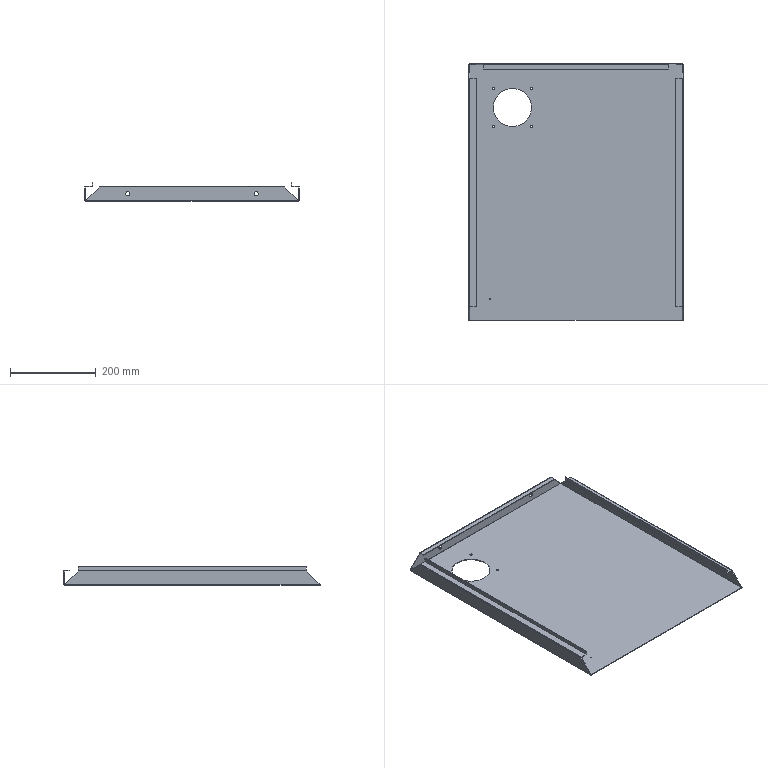Part | SolidWorks | features EdgeFlange 5, ICE 3, FlatPattern 1, MirrorPattern 1, SMBaseFlange 1, SheetMetal 1 | 1 solid | 78 faces | box 500 x 598.5 x 43.5 mm | volume 564648 mm3 | plane 54 | cylinder 24 | commonest cylinder face diameters 3 x8 5 x8 10 x4 2.5 x2 89 x2